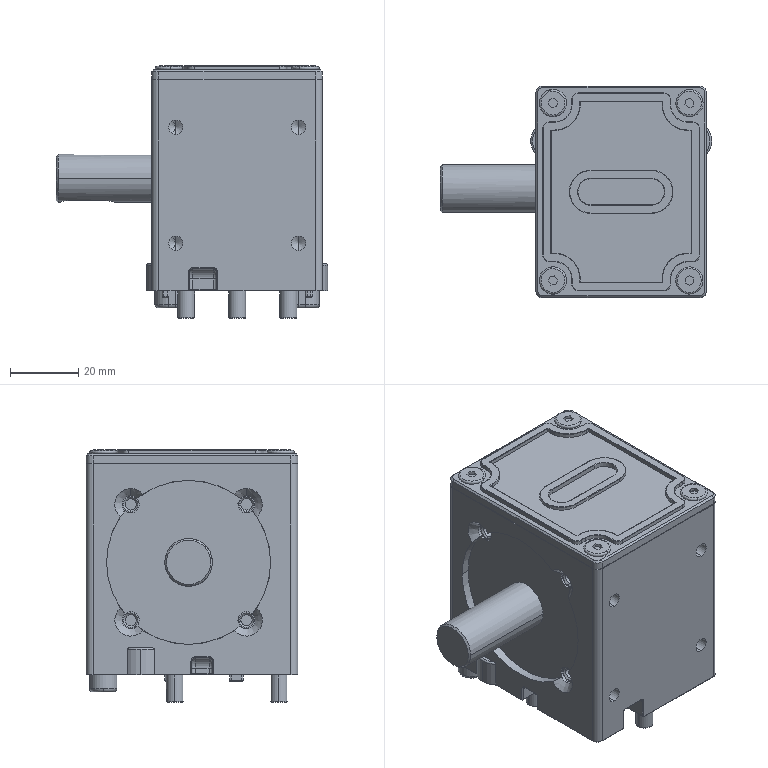Part | SolidWorks | features BaseBody 13, ICE 3, Chamfer 2 | 13 solids | 1006 faces | box 79.5 x 62 x 74 mm | volume 200359 mm3 | plane 444 | cylinder 309 | cone 177 | torus 56 | sphere 12 | spline 8 | commonest cylinder face diameters 2 x51 5 x37 1 x24 4 x24 0.2 x18 0.6 x16